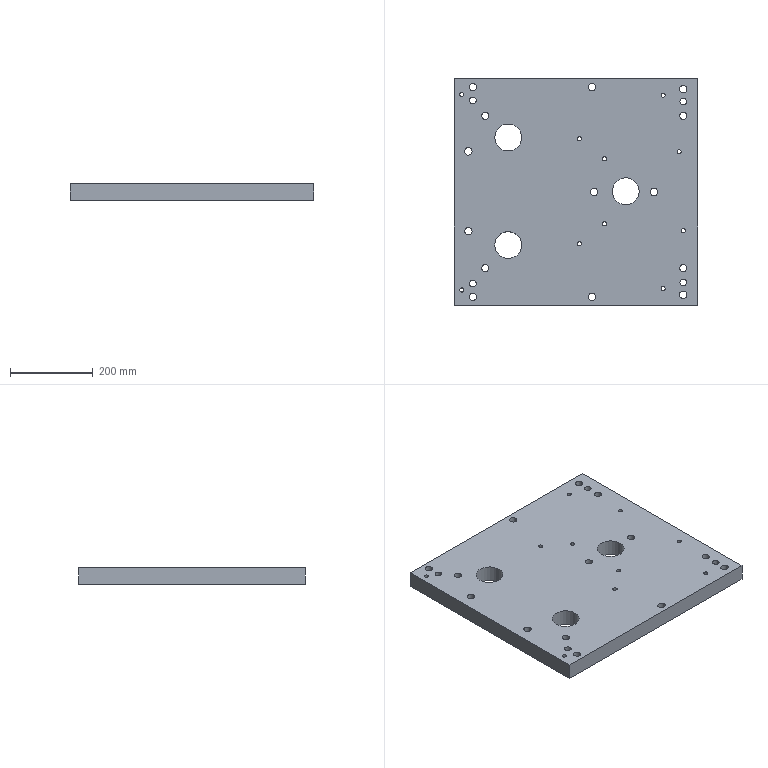Part | STEP file | lll_id2982_x_t | 1 solid | 179 faces | box 590 x 548 x 40 mm | volume 12179151 mm3 | cylinder 102 | cone 61 | plane 16 | commonest cylinder face diameters 8.505 x36 8.506 x25 10 x10 18.009 x10 26.007 x10 16 x4